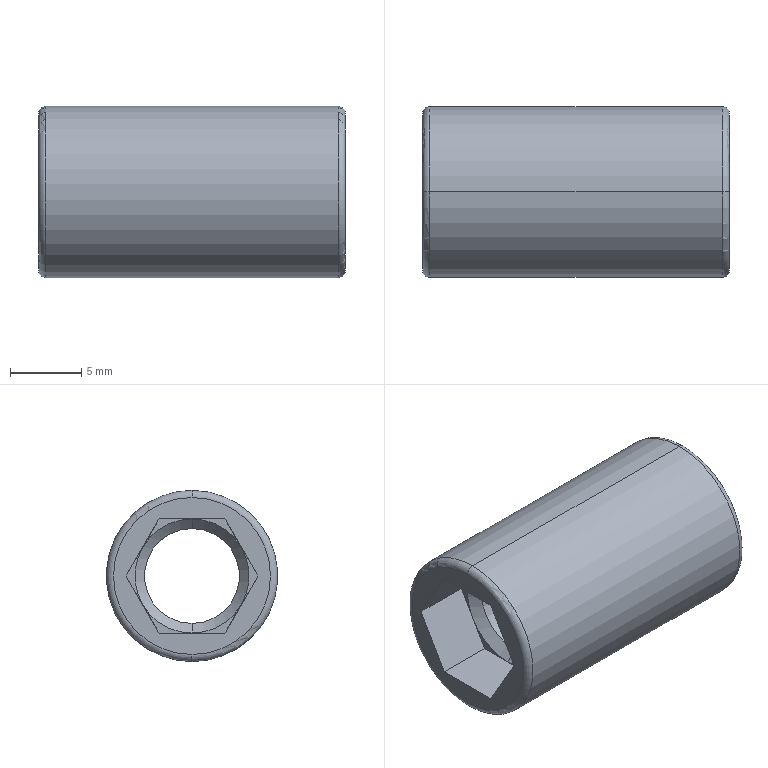Part | STEP file | JSI63_2 | 1 solid | 26 faces | box 21.5 x 12 x 12 mm | volume 1588 mm3 | plane 14 | cone 4 | cylinder 4 | torus 4 | commonest cylinder face diameters 6.647 x2 12 x2